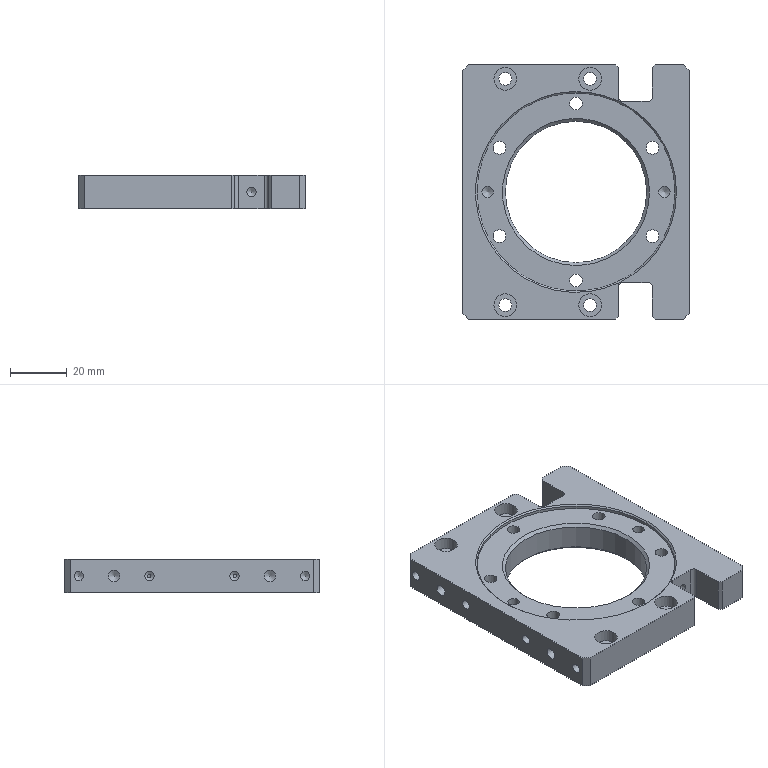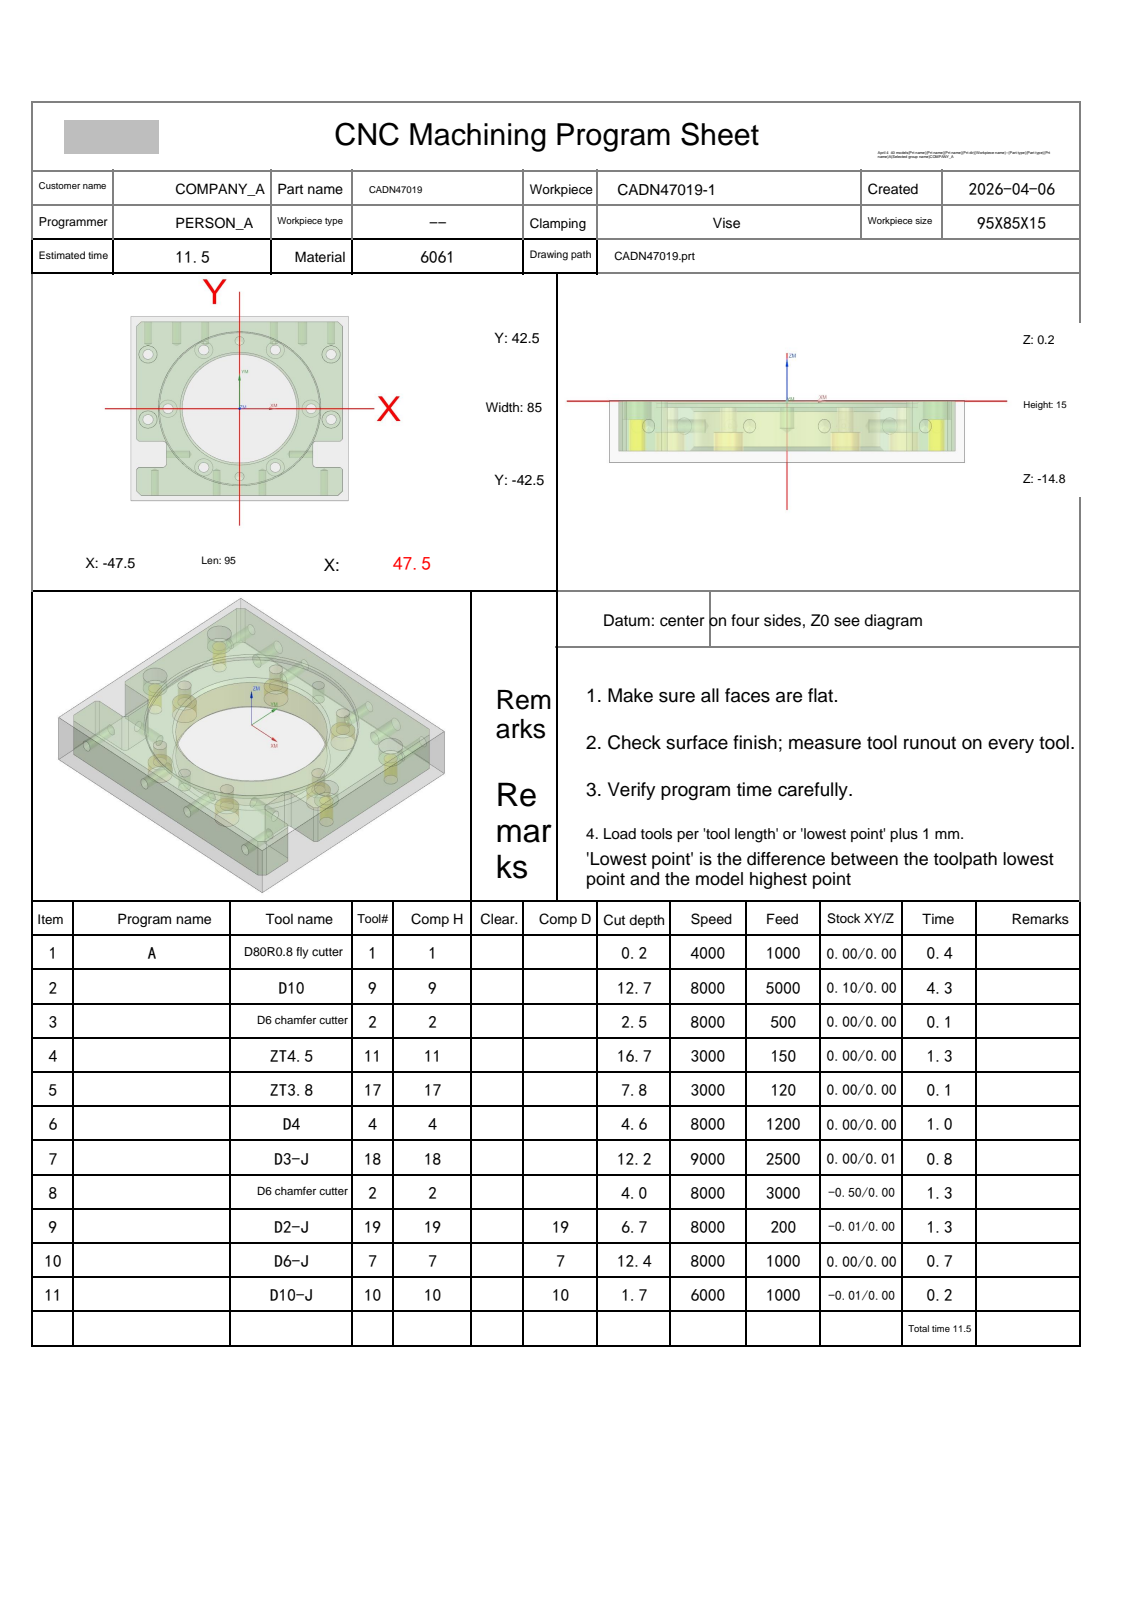NC program | NX | posted by the shop | part box 80 x 90 x 12 mm
Lines 1 to 1818 of 6628, first 1268 of 1816 lines:
%
O0001
(Machine time: 13.74 MIN)
(===Total Tool:10===)
(T1=D80R0.8 fly cutter D=80.  R=0.8  D-  H01 Z=-0.   )
(T9=D10     D=10.  R=0.   D-  H09 Z=-12.5 )
(T2=D6 chamfer cutter   D=6.   R=0.   D-  H02 Z=-3.8  )
(T11=ZT4.5  D=4.5  DR_a=118 D-  H11 Z=-16.5 )
(T17=ZT3.8  D=3.8  DR_a=118 D-  H17 Z=-7.6  )
(T4=D4      D=4.   R=0.   D4  H04 Z=-4.4  )
(T18=D3-J   D=3.   R=0.   D-  H18 Z=-11.95)
(T19=D2-J   D=2.   R=0.   D19 H19 Z=-6.5  )
(T7=D6-J    D=6.   R=0.   D7  H07 Z=-12.2 )
(T10=D10-J  D=10.  R=0.   D10 H10 Z=-1.5  )
G80 G90 G17 G49 G40
G91 G28 Z0
M01
N1 T01 M06
(D80R0.8 fly cutter  D=80. R=0.8 H=01 ce=0.00 di=0.00)
G00 G90 G54 X-90. Y26.667 M03 S4000
G43 H01 Z20.
M08
Z2.
G01 Z0.0 F1000.
X-85.
X85.
Y-26.667
X-85.
X-90.
Z2.
G00 Z20.
G91 G28 Z0.0
M05
M09
G91 G28 Z0.0
M01
N2 T09 M06
(D10  D=10. R=0. H=09 ce=0.10 di=0.00)
G00 G90 G54 X0.0 Y-45.1 M03 S8000
G43 H09 Z20.
M08
Z.5
G01 X-43. Z.416 F5000.
G02 X-46.606 Y-43.606 Z.409 I0.0 J5.1
G01 X-48.606 Y-41.606 Z.403
G02 X-50.1 Y-38. Z.395 I3.606 J3.606
G01 Y-28. Z.376
G02 X-48.606 Y-24.394 Z.368 I5.1 J0.0
G01 X-47.606 Y-23.394 Z.365
G02 X-44. Y-21.9 Z.358 I3.606 J-3.606
G01 X-37.1 Z.344
Y-20.1 Z.341
X-44. Z.327
G02 X-47.606 Y-18.606 Z.319 I0.0 J5.1
G01 X-48.606 Y-17.606 Z.317
G02 X-50.1 Y-14. Z.309 I3.606 J3.606
G01 Y38. Z.208
G02 X-48.606 Y41.606 Z.2 I5.1 J0.0
G01 X-46.606 Y43.606 Z.195
G02 X-43. Y45.1 Z.187 I3.606 J-3.606
G01 X43. Z.02
G02 X46.606 Y43.606 Z.012 I0.0 J-5.1
G01 X48.606 Y41.606 Z.006
G02 X50.1 Y38. Z-.002 I-3.606 J-3.606
G01 Y-14. Z-.103
G02 X48.606 Y-17.606 Z-.11 I-5.1 J0.0
G01 X47.606 Y-18.606 Z-.113
G02 X44.357 Y-20.087 Z-.12 I-3.606 J3.606
X44. Y-20.1 Z-.121 I-.357 J5.087
G01 X37.1 Z-.134
Y-21.9 Z-.138
X44. Z-.151
G02 X47.606 Y-23.394 Z-.159 I0.0 J-5.1
G01 X48.606 Y-24.394 Z-.162
G02 X50.1 Y-28. Z-.17 I-3.606 J-3.606
G01 Y-38. Z-.189
G02 X48.606 Y-41.606 Z-.197 I-5.1 J0.0
G01 X46.606 Y-43.606 Z-.202
G02 X43. Y-45.1 Z-.21 I-3.606 J3.606
G01 X-43. Z-.377
G02 X-46.606 Y-43.606 Z-.385 I0.0 J5.1
G01 X-48.606 Y-41.606 Z-.391
G02 X-50.1 Y-38. Z-.398 I3.606 J3.606
G01 Y-28. Z-.418
G02 X-48.606 Y-24.394 Z-.426 I5.1 J0.0
G01 X-47.606 Y-23.394 Z-.428
G02 X-44. Y-21.9 Z-.436 I3.606 J-3.606
G01 X-37.1 Z-.45
Y-20.1 Z-.453
X-44. Z-.467
G02 X-47.606 Y-18.606 Z-.474 I0.0 J5.1
G01 X-48.606 Y-17.606 Z-.477
G02 X-50.1 Y-14. Z-.485 I3.606 J3.606
G01 Y38. Z-.586
G02 X-48.606 Y41.606 Z-.594 I5.1 J0.0
G01 X-46.606 Y43.606 Z-.599
G02 X-43. Y45.1 Z-.607 I3.606 J-3.606
G01 X43. Z-.774
G02 X46.606 Y43.606 Z-.782 I0.0 J-5.1
G01 X48.606 Y41.606 Z-.788
G02 X50.1 Y38. Z-.795 I-3.606 J-3.606
G01 Y-14. Z-.896
G02 X48.606 Y-17.606 Z-.904 I-5.1 J0.0
G01 X47.606 Y-18.606 Z-.907
G02 X44.357 Y-20.087 Z-.914 I-3.606 J3.606
X44. Y-20.1 Z-.915 I-.357 J5.087
G01 X37.1 Z-.928
Y-21.9 Z-.932
X44. Z-.945
G02 X47.606 Y-23.394 Z-.953 I0.0 J-5.1
G01 X48.606 Y-24.394 Z-.956
G02 X50.1 Y-28. Z-.963 I-3.606 J-3.606
G01 Y-38. Z-.983
G02 X48.606 Y-41.606 Z-.991 I-5.1 J0.0
G01 X46.606 Y-43.606 Z-.996
G02 X43. Y-45.1 Z-1.004 I-3.606 J3.606
G01 X-43. Z-1.171
G02 X-46.606 Y-43.606 Z-1.179 I0.0 J5.1
G01 X-48.606 Y-41.606 Z-1.184
G02 X-50.1 Y-38. Z-1.192 I3.606 J3.606
G01 Y-28. Z-1.212
G02 X-48.606 Y-24.394 Z-1.219 I5.1 J0.0
G01 X-47.606 Y-23.394 Z-1.222
G02 X-44. Y-21.9 Z-1.23 I3.606 J-3.606
G01 X-37.1 Z-1.243
Y-20.1 Z-1.247
X-44. Z-1.26
G02 X-47.606 Y-18.606 Z-1.268 I0.0 J5.1
G01 X-48.606 Y-17.606 Z-1.271
G02 X-50.1 Y-14. Z-1.279 I3.606 J3.606
G01 Y38. Z-1.38
G02 X-48.606 Y41.606 Z-1.387 I5.1 J0.0
G01 X-46.606 Y43.606 Z-1.393
G02 X-43. Y45.1 Z-1.401 I3.606 J-3.606
G01 X43. Z-1.568
G02 X46.606 Y43.606 Z-1.576 I0.0 J-5.1
G01 X48.606 Y41.606 Z-1.581
G02 X50.1 Y38. Z-1.589 I-3.606 J-3.606
G01 Y-14. Z-1.69
G02 X48.606 Y-17.606 Z-1.698 I-5.1 J0.0
G01 X47.606 Y-18.606 Z-1.701
G02 X44.357 Y-20.087 Z-1.708 I-3.606 J3.606
X44. Y-20.1 Z-1.708 I-.357 J5.087
G01 X37.1 Z-1.722
Y-21.9 Z-1.725
X44. Z-1.739
G02 X47.606 Y-23.394 Z-1.747 I0.0 J-5.1
G01 X48.606 Y-24.394 Z-1.749
G02 X50.1 Y-28. Z-1.757 I-3.606 J-3.606
G01 Y-38. Z-1.777
G02 X48.606 Y-41.606 Z-1.784 I-5.1 J0.0
G01 X46.606 Y-43.606 Z-1.79
G02 X43. Y-45.1 Z-1.798 I-3.606 J3.606
G01 X-43. Z-1.965
G02 X-46.606 Y-43.606 Z-1.973 I0.0 J5.1
G01 X-48.606 Y-41.606 Z-1.978
G02 X-50.1 Y-38. Z-1.986 I3.606 J3.606
G01 Y-28. Z-2.005
G02 X-48.606 Y-24.394 Z-2.013 I5.1 J0.0
G01 X-47.606 Y-23.394 Z-2.016
G02 X-44. Y-21.9 Z-2.024 I3.606 J-3.606
G01 X-37.1 Z-2.037
Y-20.1 Z-2.041
X-44. Z-2.054
G02 X-47.606 Y-18.606 Z-2.062 I0.0 J5.1
G01 X-48.606 Y-17.606 Z-2.065
G02 X-50.1 Y-14. Z-2.072 I3.606 J3.606
G01 Y38. Z-2.173
G02 X-48.606 Y41.606 Z-2.181 I5.1 J0.0
G01 X-46.606 Y43.606 Z-2.187
G02 X-43. Y45.1 Z-2.195 I3.606 J-3.606
G01 X43. Z-2.362
G02 X46.606 Y43.606 Z-2.37 I0.0 J-5.1
G01 X48.606 Y41.606 Z-2.375
G02 X50.1 Y38. Z-2.383 I-3.606 J-3.606
G01 Y-14. Z-2.484
G02 X48.606 Y-17.606 Z-2.492 I-5.1 J0.0
G01 X47.606 Y-18.606 Z-2.494
G02 X44.357 Y-20.087 Z-2.502 I-3.606 J3.606
X44. Y-20.1 Z-2.502 I-.357 J5.087
G01 X37.1 Z-2.516
Y-21.9 Z-2.519
X44. Z-2.533
G02 X47.606 Y-23.394 Z-2.54 I0.0 J-5.1
G01 X48.606 Y-24.394 Z-2.543
G02 X50.1 Y-28. Z-2.551 I-3.606 J-3.606
G01 Y-38. Z-2.57
G02 X48.606 Y-41.606 Z-2.578 I-5.1 J0.0
G01 X46.606 Y-43.606 Z-2.584
G02 X43. Y-45.1 Z-2.591 I-3.606 J3.606
G01 X-43. Z-2.759
G02 X-46.606 Y-43.606 Z-2.766 I0.0 J5.1
G01 X-48.606 Y-41.606 Z-2.772
G02 X-50.1 Y-38. Z-2.78 I3.606 J3.606
G01 Y-28. Z-2.799
G02 X-48.606 Y-24.394 Z-2.807 I5.1 J0.0
G01 X-47.606 Y-23.394 Z-2.81
G02 X-44. Y-21.9 Z-2.817 I3.606 J-3.606
G01 X-37.1 Z-2.831
Y-20.1 Z-2.834
X-44. Z-2.848
G02 X-47.606 Y-18.606 Z-2.856 I0.0 J5.1
G01 X-48.606 Y-17.606 Z-2.858
G02 X-50.1 Y-14. Z-2.866 I3.606 J3.606
G01 Y38. Z-2.967
G02 X-48.606 Y41.606 Z-2.975 I5.1 J0.0
G01 X-46.606 Y43.606 Z-2.98
G02 X-43. Y45.1 Z-2.988 I3.606 J-3.606
G01 X43. Z-3.155
G02 X46.606 Y43.606 Z-3.163 I0.0 J-5.1
G01 X48.606 Y41.606 Z-3.169
G02 X50.1 Y38. Z-3.177 I-3.606 J-3.606
G01 Y-14. Z-3.278
G02 X48.606 Y-17.606 Z-3.285 I-5.1 J0.0
G01 X47.606 Y-18.606 Z-3.288
G02 X44.357 Y-20.087 Z-3.295 I-3.606 J3.606
X44. Y-20.1 Z-3.296 I-.357 J5.087
G01 X37.1 Z-3.309
Y-21.9 Z-3.313
X44. Z-3.326
G02 X47.606 Y-23.394 Z-3.334 I0.0 J-5.1
G01 X48.606 Y-24.394 Z-3.337
G02 X50.1 Y-28. Z-3.345 I-3.606 J-3.606
G01 Y-38. Z-3.364
G02 X48.606 Y-41.606 Z-3.372 I-5.1 J0.0
G01 X46.606 Y-43.606 Z-3.377
G02 X43. Y-45.1 Z-3.385 I-3.606 J3.606
G01 X-43. Z-3.552
G02 X-46.606 Y-43.606 Z-3.56 I0.0 J5.1
G01 X-48.606 Y-41.606 Z-3.566
G02 X-50.1 Y-38. Z-3.573 I3.606 J3.606
G01 Y-28. Z-3.593
G02 X-48.606 Y-24.394 Z-3.601 I5.1 J0.0
G01 X-47.606 Y-23.394 Z-3.603
G02 X-44. Y-21.9 Z-3.611 I3.606 J-3.606
G01 X-37.1 Z-3.625
Y-20.1 Z-3.628
X-44. Z-3.642
G02 X-47.606 Y-18.606 Z-3.649 I0.0 J5.1
G01 X-48.606 Y-17.606 Z-3.652
G02 X-50.1 Y-14. Z-3.66 I3.606 J3.606
G01 Y38. Z-3.761
G02 X-48.606 Y41.606 Z-3.769 I5.1 J0.0
G01 X-46.606 Y43.606 Z-3.774
G02 X-43. Y45.1 Z-3.782 I3.606 J-3.606
G01 X43. Z-3.949
G02 X46.606 Y43.606 Z-3.957 I0.0 J-5.1
G01 X48.606 Y41.606 Z-3.963
G02 X50.1 Y38. Z-3.97 I-3.606 J-3.606
G01 Y-14. Z-4.071
G02 X48.606 Y-17.606 Z-4.079 I-5.1 J0.0
G01 X47.606 Y-18.606 Z-4.082
G02 X44.357 Y-20.087 Z-4.089 I-3.606 J3.606
X44. Y-20.1 Z-4.09 I-.357 J5.087
G01 X37.1 Z-4.103
Y-21.9 Z-4.107
X44. Z-4.12
G02 X47.606 Y-23.394 Z-4.128 I0.0 J-5.1
G01 X48.606 Y-24.394 Z-4.131
G02 X50.1 Y-28. Z-4.138 I-3.606 J-3.606
G01 Y-38. Z-4.158
G02 X48.606 Y-41.606 Z-4.166 I-5.1 J0.0
G01 X46.606 Y-43.606 Z-4.171
G02 X43. Y-45.1 Z-4.179 I-3.606 J3.606
G01 X-43. Z-4.346
G02 X-46.606 Y-43.606 Z-4.354 I0.0 J5.1
G01 X-48.606 Y-41.606 Z-4.359
G02 X-50.1 Y-38. Z-4.367 I3.606 J3.606
G01 Y-28. Z-4.387
G02 X-48.606 Y-24.394 Z-4.394 I5.1 J0.0
G01 X-47.606 Y-23.394 Z-4.397
G02 X-44. Y-21.9 Z-4.405 I3.606 J-3.606
G01 X-37.1 Z-4.418
Y-20.1 Z-4.422
X-44. Z-4.435
G02 X-47.606 Y-18.606 Z-4.443 I0.0 J5.1
G01 X-48.606 Y-17.606 Z-4.446
G02 X-50.1 Y-14. Z-4.454 I3.606 J3.606
G01 Y38. Z-4.555
G02 X-48.606 Y41.606 Z-4.562 I5.1 J0.0
G01 X-46.606 Y43.606 Z-4.568
G02 X-43. Y45.1 Z-4.576 I3.606 J-3.606
G01 X43. Z-4.743
G02 X46.606 Y43.606 Z-4.751 I0.0 J-5.1
G01 X48.606 Y41.606 Z-4.756
G02 X50.1 Y38. Z-4.764 I-3.606 J-3.606
G01 Y-14. Z-4.865
G02 X48.606 Y-17.606 Z-4.873 I-5.1 J0.0
G01 X47.606 Y-18.606 Z-4.876
G02 X44.357 Y-20.087 Z-4.883 I-3.606 J3.606
X44. Y-20.1 Z-4.883 I-.357 J5.087
G01 X37.1 Z-4.897
Y-21.9 Z-4.9
X44. Z-4.914
G02 X47.606 Y-23.394 Z-4.922 I0.0 J-5.1
G01 X48.606 Y-24.394 Z-4.924
G02 X50.1 Y-28. Z-4.932 I-3.606 J-3.606
G01 Y-38. Z-4.952
G02 X48.606 Y-41.606 Z-4.959 I-5.1 J0.0
G01 X46.606 Y-43.606 Z-4.965
G02 X43. Y-45.1 Z-4.973 I-3.606 J3.606
G01 X-43. Z-5.14
G02 X-46.606 Y-43.606 Z-5.148 I0.0 J5.1
G01 X-48.606 Y-41.606 Z-5.153
G02 X-50.1 Y-38. Z-5.161 I3.606 J3.606
G01 Y-28. Z-5.18
G02 X-48.606 Y-24.394 Z-5.188 I5.1 J0.0
G01 X-47.606 Y-23.394 Z-5.191
G02 X-44. Y-21.9 Z-5.199 I3.606 J-3.606
G01 X-37.1 Z-5.212
Y-20.1 Z-5.216
X-44. Z-5.229
G02 X-47.606 Y-18.606 Z-5.237 I0.0 J5.1
G01 X-48.606 Y-17.606 Z-5.24
G02 X-50.1 Y-14. Z-5.247 I3.606 J3.606
G01 Y38. Z-5.348
G02 X-48.606 Y41.606 Z-5.356 I5.1 J0.0
G01 X-46.606 Y43.606 Z-5.362
G02 X-43. Y45.1 Z-5.37 I3.606 J-3.606
G01 X43. Z-5.537
G02 X46.606 Y43.606 Z-5.545 I0.0 J-5.1
G01 X48.606 Y41.606 Z-5.55
G02 X50.1 Y38. Z-5.558 I-3.606 J-3.606
G01 Y-14. Z-5.659
G02 X48.606 Y-17.606 Z-5.667 I-5.1 J0.0
G01 X47.606 Y-18.606 Z-5.669
G02 X44.357 Y-20.087 Z-5.677 I-3.606 J3.606
X44. Y-20.1 Z-5.677 I-.357 J5.087
G01 X37.1 Z-5.691
Y-21.9 Z-5.694
X44. Z-5.708
G02 X47.606 Y-23.394 Z-5.715 I0.0 J-5.1
G01 X48.606 Y-24.394 Z-5.718
G02 X50.1 Y-28. Z-5.726 I-3.606 J-3.606
G01 Y-38. Z-5.745
G02 X48.606 Y-41.606 Z-5.753 I-5.1 J0.0
G01 X46.606 Y-43.606 Z-5.759
G02 X43. Y-45.1 Z-5.766 I-3.606 J3.606
G01 X-43. Z-5.934
G02 X-46.606 Y-43.606 Z-5.941 I0.0 J5.1
G01 X-48.606 Y-41.606 Z-5.947
G02 X-50.1 Y-38. Z-5.955 I3.606 J3.606
G01 Y-28. Z-5.974
G02 X-48.606 Y-24.394 Z-5.982 I5.1 J0.0
G01 X-47.606 Y-23.394 Z-5.985
G02 X-44. Y-21.9 Z-5.992 I3.606 J-3.606
G01 X-37.1 Z-6.006
Y-20.1 Z-6.009
X-44. Z-6.023
G02 X-47.606 Y-18.606 Z-6.031 I0.0 J5.1
G01 X-48.606 Y-17.606 Z-6.033
G02 X-50.1 Y-14. Z-6.041 I3.606 J3.606
G01 Y38. Z-6.142
G02 X-48.606 Y41.606 Z-6.15 I5.1 J0.0
G01 X-46.606 Y43.606 Z-6.155
G02 X-43. Y45.1 Z-6.163 I3.606 J-3.606
G01 X43. Z-6.33
G02 X46.606 Y43.606 Z-6.338 I0.0 J-5.1
G01 X48.606 Y41.606 Z-6.344
G02 X50.1 Y38. Z-6.352 I-3.606 J-3.606
G01 Y-14. Z-6.453
G02 X48.606 Y-17.606 Z-6.46 I-5.1 J0.0
G01 X47.606 Y-18.606 Z-6.463
G02 X44.357 Y-20.087 Z-6.47 I-3.606 J3.606
X44. Y-20.1 Z-6.471 I-.357 J5.087
G01 X37.1 Z-6.484
Y-21.9 Z-6.488
X44. Z-6.501
G02 X47.606 Y-23.394 Z-6.509 I0.0 J-5.1
G01 X48.606 Y-24.394 Z-6.512
G02 X50.1 Y-28. Z-6.52 I-3.606 J-3.606
G01 Y-38. Z-6.539
G02 X48.606 Y-41.606 Z-6.547 I-5.1 J0.0
G01 X46.606 Y-43.606 Z-6.552
G02 X43. Y-45.1 Z-6.56 I-3.606 J3.606
G01 X-43. Z-6.727
G02 X-46.606 Y-43.606 Z-6.735 I0.0 J5.1
G01 X-48.606 Y-41.606 Z-6.741
G02 X-50.1 Y-38. Z-6.748 I3.606 J3.606
G01 Y-28. Z-6.768
G02 X-48.606 Y-24.394 Z-6.776 I5.1 J0.0
G01 X-47.606 Y-23.394 Z-6.778
G02 X-44. Y-21.9 Z-6.786 I3.606 J-3.606
G01 X-37.1 Z-6.8
Y-20.1 Z-6.803
X-44. Z-6.817
G02 X-47.606 Y-18.606 Z-6.824 I0.0 J5.1
G01 X-48.606 Y-17.606 Z-6.827
G02 X-50.1 Y-14. Z-6.835 I3.606 J3.606
G01 Y38. Z-6.936
G02 X-48.606 Y41.606 Z-6.944 I5.1 J0.0
G01 X-46.606 Y43.606 Z-6.949
G02 X-43. Y45.1 Z-6.957 I3.606 J-3.606
G01 X43. Z-7.124
G02 X46.606 Y43.606 Z-7.132 I0.0 J-5.1
G01 X48.606 Y41.606 Z-7.138
G02 X50.1 Y38. Z-7.145 I-3.606 J-3.606
G01 Y-14. Z-7.246
G02 X48.606 Y-17.606 Z-7.254 I-5.1 J0.0
G01 X47.606 Y-18.606 Z-7.257
G02 X44.357 Y-20.087 Z-7.264 I-3.606 J3.606
X44. Y-20.1 Z-7.265 I-.357 J5.087
G01 X37.1 Z-7.278
Y-21.9 Z-7.282
X44. Z-7.295
G02 X47.606 Y-23.394 Z-7.303 I0.0 J-5.1
G01 X48.606 Y-24.394 Z-7.306
G02 X50.1 Y-28. Z-7.313 I-3.606 J-3.606
G01 Y-38. Z-7.333
G02 X48.606 Y-41.606 Z-7.341 I-5.1 J0.0
G01 X46.606 Y-43.606 Z-7.346
G02 X43. Y-45.1 Z-7.354 I-3.606 J3.606
G01 X-43. Z-7.521
G02 X-46.606 Y-43.606 Z-7.529 I0.0 J5.1
G01 X-48.606 Y-41.606 Z-7.534
G02 X-50.1 Y-38. Z-7.542 I3.606 J3.606
G01 Y-28. Z-7.562
G02 X-48.606 Y-24.394 Z-7.569 I5.1 J0.0
G01 X-47.606 Y-23.394 Z-7.572
G02 X-44. Y-21.9 Z-7.58 I3.606 J-3.606
G01 X-37.1 Z-7.593
Y-20.1 Z-7.597
X-44. Z-7.61
G02 X-47.606 Y-18.606 Z-7.618 I0.0 J5.1
G01 X-48.606 Y-17.606 Z-7.621
G02 X-50.1 Y-14. Z-7.629 I3.606 J3.606
G01 Y38. Z-7.73
G02 X-48.606 Y41.606 Z-7.737 I5.1 J0.0
G01 X-46.606 Y43.606 Z-7.743
G02 X-43. Y45.1 Z-7.751 I3.606 J-3.606
G01 X43. Z-7.918
G02 X46.606 Y43.606 Z-7.926 I0.0 J-5.1
G01 X48.606 Y41.606 Z-7.931
G02 X50.1 Y38. Z-7.939 I-3.606 J-3.606
G01 Y-14. Z-8.04
G02 X48.606 Y-17.606 Z-8.048 I-5.1 J0.0
G01 X47.606 Y-18.606 Z-8.051
G02 X44.357 Y-20.087 Z-8.058 I-3.606 J3.606
X44. Y-20.1 Z-8.058 I-.357 J5.087
G01 X37.1 Z-8.072
Y-21.9 Z-8.075
X44. Z-8.089
G02 X47.606 Y-23.394 Z-8.097 I0.0 J-5.1
G01 X48.606 Y-24.394 Z-8.099
G02 X50.1 Y-28. Z-8.107 I-3.606 J-3.606
G01 Y-38. Z-8.127
G02 X48.606 Y-41.606 Z-8.134 I-5.1 J0.0
G01 X46.606 Y-43.606 Z-8.14
G02 X43. Y-45.1 Z-8.148 I-3.606 J3.606
G01 X-43. Z-8.315
G02 X-46.606 Y-43.606 Z-8.323 I0.0 J5.1
G01 X-48.606 Y-41.606 Z-8.328
G02 X-50.1 Y-38. Z-8.336 I3.606 J3.606
G01 Y-28. Z-8.355
G02 X-48.606 Y-24.394 Z-8.363 I5.1 J0.0
G01 X-47.606 Y-23.394 Z-8.366
G02 X-44. Y-21.9 Z-8.374 I3.606 J-3.606
G01 X-37.1 Z-8.387
Y-20.1 Z-8.391
X-44. Z-8.404
G02 X-47.606 Y-18.606 Z-8.412 I0.0 J5.1
G01 X-48.606 Y-17.606 Z-8.415
G02 X-50.1 Y-14. Z-8.422 I3.606 J3.606
G01 Y38. Z-8.523
G02 X-48.606 Y41.606 Z-8.531 I5.1 J0.0
G01 X-46.606 Y43.606 Z-8.537
G02 X-43. Y45.1 Z-8.545 I3.606 J-3.606
G01 X43. Z-8.712
G02 X46.606 Y43.606 Z-8.72 I0.0 J-5.1
G01 X48.606 Y41.606 Z-8.725
G02 X50.1 Y38. Z-8.733 I-3.606 J-3.606
G01 Y-14. Z-8.834
G02 X48.606 Y-17.606 Z-8.842 I-5.1 J0.0
G01 X47.606 Y-18.606 Z-8.844
G02 X44.357 Y-20.087 Z-8.852 I-3.606 J3.606
X44. Y-20.1 Z-8.852 I-.357 J5.087
G01 X37.1 Z-8.866
Y-21.9 Z-8.869
X44. Z-8.883
G02 X47.606 Y-23.394 Z-8.89 I0.0 J-5.1
G01 X48.606 Y-24.394 Z-8.893
G02 X50.1 Y-28. Z-8.901 I-3.606 J-3.606
G01 Y-38. Z-8.92
G02 X48.606 Y-41.606 Z-8.928 I-5.1 J0.0
G01 X46.606 Y-43.606 Z-8.934
G02 X43. Y-45.1 Z-8.941 I-3.606 J3.606
G01 X-43. Z-9.109
G02 X-46.606 Y-43.606 Z-9.116 I0.0 J5.1
G01 X-48.606 Y-41.606 Z-9.122
G02 X-50.1 Y-38. Z-9.13 I3.606 J3.606
G01 Y-28. Z-9.149
G02 X-48.606 Y-24.394 Z-9.157 I5.1 J0.0
G01 X-47.606 Y-23.394 Z-9.16
G02 X-44. Y-21.9 Z-9.167 I3.606 J-3.606
G01 X-37.1 Z-9.181
Y-20.1 Z-9.184
X-44. Z-9.198
G02 X-47.606 Y-18.606 Z-9.206 I0.0 J5.1
G01 X-48.606 Y-17.606 Z-9.208
G02 X-50.1 Y-14. Z-9.216 I3.606 J3.606
G01 Y38. Z-9.317
G02 X-48.606 Y41.606 Z-9.325 I5.1 J0.0
G01 X-46.606 Y43.606 Z-9.33
G02 X-43. Y45.1 Z-9.338 I3.606 J-3.606
G01 X43. Z-9.505
G02 X46.606 Y43.606 Z-9.513 I0.0 J-5.1
G01 X48.606 Y41.606 Z-9.519
G02 X50.1 Y38. Z-9.527 I-3.606 J-3.606
G01 Y-14. Z-9.628
G02 X48.606 Y-17.606 Z-9.635 I-5.1 J0.0
G01 X47.606 Y-18.606 Z-9.638
G02 X44.357 Y-20.087 Z-9.645 I-3.606 J3.606
X44. Y-20.1 Z-9.646 I-.357 J5.087
G01 X37.1 Z-9.659
Y-21.9 Z-9.663
X44. Z-9.676
G02 X47.606 Y-23.394 Z-9.684 I0.0 J-5.1
G01 X48.606 Y-24.394 Z-9.687
G02 X50.1 Y-28. Z-9.695 I-3.606 J-3.606
G01 Y-38. Z-9.714
G02 X48.606 Y-41.606 Z-9.722 I-5.1 J0.0
G01 X46.606 Y-43.606 Z-9.727
G02 X43. Y-45.1 Z-9.735 I-3.606 J3.606
G01 X-43. Z-9.902
G02 X-46.606 Y-43.606 Z-9.91 I0.0 J5.1
G01 X-48.606 Y-41.606 Z-9.916
G02 X-50.1 Y-38. Z-9.923 I3.606 J3.606
G01 Y-28. Z-9.943
G02 X-48.606 Y-24.394 Z-9.951 I5.1 J0.0
G01 X-47.606 Y-23.394 Z-9.953
G02 X-44. Y-21.9 Z-9.961 I3.606 J-3.606
G01 X-37.1 Z-9.975
Y-20.1 Z-9.978
X-44. Z-9.992
G02 X-47.606 Y-18.606 Z-9.999 I0.0 J5.1
G01 X-48.606 Y-17.606 Z-10.002
G02 X-50.1 Y-14. Z-10.01 I3.606 J3.606
G01 Y38. Z-10.111
G02 X-48.606 Y41.606 Z-10.119 I5.1 J0.0
G01 X-46.606 Y43.606 Z-10.124
G02 X-43. Y45.1 Z-10.132 I3.606 J-3.606
G01 X43. Z-10.299
G02 X46.606 Y43.606 Z-10.307 I0.0 J-5.1
G01 X48.606 Y41.606 Z-10.313
G02 X50.1 Y38. Z-10.32 I-3.606 J-3.606
G01 Y-14. Z-10.421
G02 X48.606 Y-17.606 Z-10.429 I-5.1 J0.0
G01 X47.606 Y-18.606 Z-10.432
G02 X44.357 Y-20.087 Z-10.439 I-3.606 J3.606
X44. Y-20.1 Z-10.44 I-.357 J5.087
G01 X37.1 Z-10.453
Y-21.9 Z-10.457
X44. Z-10.47
G02 X47.606 Y-23.394 Z-10.478 I0.0 J-5.1
G01 X48.606 Y-24.394 Z-10.481
G02 X50.1 Y-28. Z-10.488 I-3.606 J-3.606
G01 Y-38. Z-10.508
G02 X48.606 Y-41.606 Z-10.516 I-5.1 J0.0
G01 X46.606 Y-43.606 Z-10.521
G02 X43. Y-45.1 Z-10.529 I-3.606 J3.606
G01 X-43. Z-10.696
G02 X-46.606 Y-43.606 Z-10.704 I0.0 J5.1
G01 X-48.606 Y-41.606 Z-10.709
G02 X-50.1 Y-38. Z-10.717 I3.606 J3.606
G01 Y-28. Z-10.737
G02 X-48.606 Y-24.394 Z-10.744 I5.1 J0.0
G01 X-47.606 Y-23.394 Z-10.747
G02 X-44. Y-21.9 Z-10.755 I3.606 J-3.606
G01 X-37.1 Z-10.768
Y-20.1 Z-10.772
X-44. Z-10.785
G02 X-47.606 Y-18.606 Z-10.793 I0.0 J5.1
G01 X-48.606 Y-17.606 Z-10.796
G02 X-50.1 Y-14. Z-10.804 I3.606 J3.606
G01 Y38. Z-10.905
G02 X-48.606 Y41.606 Z-10.912 I5.1 J0.0
G01 X-46.606 Y43.606 Z-10.918
G02 X-43. Y45.1 Z-10.926 I3.606 J-3.606
G01 X43. Z-11.093
G02 X46.606 Y43.606 Z-11.101 I0.0 J-5.1
G01 X48.606 Y41.606 Z-11.106
G02 X50.1 Y38. Z-11.114 I-3.606 J-3.606
G01 Y-14. Z-11.215
G02 X48.606 Y-17.606 Z-11.223 I-5.1 J0.0
G01 X47.606 Y-18.606 Z-11.226
G02 X44.357 Y-20.087 Z-11.233 I-3.606 J3.606
X44. Y-20.1 Z-11.233 I-.357 J5.087
G01 X37.1 Z-11.247
Y-21.9 Z-11.25
X44. Z-11.264
G02 X47.606 Y-23.394 Z-11.272 I0.0 J-5.1
G01 X48.606 Y-24.394 Z-11.274
G02 X50.1 Y-28. Z-11.282 I-3.606 J-3.606
G01 Y-38. Z-11.302
G02 X48.606 Y-41.606 Z-11.309 I-5.1 J0.0
G01 X46.606 Y-43.606 Z-11.315
G02 X43. Y-45.1 Z-11.323 I-3.606 J3.606
G01 X-43. Z-11.49
G02 X-46.606 Y-43.606 Z-11.498 I0.0 J5.1
G01 X-48.606 Y-41.606 Z-11.503
G02 X-50.1 Y-38. Z-11.511 I3.606 J3.606
G01 Y-28. Z-11.53
G02 X-48.606 Y-24.394 Z-11.538 I5.1 J0.0
G01 X-47.606 Y-23.394 Z-11.541
G02 X-44. Y-21.9 Z-11.549 I3.606 J-3.606
G01 X-37.1 Z-11.562
Y-20.1 Z-11.566
X-44. Z-11.579
G02 X-47.606 Y-18.606 Z-11.587 I0.0 J5.1
G01 X-48.606 Y-17.606 Z-11.59
G02 X-50.1 Y-14. Z-11.597 I3.606 J3.606
G01 Y38. Z-11.698
G02 X-48.606 Y41.606 Z-11.706 I5.1 J0.0
G01 X-46.606 Y43.606 Z-11.712
G02 X-43. Y45.1 Z-11.72 I3.606 J-3.606
G01 X43. Z-11.887
G02 X46.606 Y43.606 Z-11.895 I0.0 J-5.1
G01 X48.606 Y41.606 Z-11.9
G02 X50.1 Y38. Z-11.908 I-3.606 J-3.606
G01 Y-14. Z-12.009
G02 X48.606 Y-17.606 Z-12.017 I-5.1 J0.0
G01 X47.606 Y-18.606 Z-12.019
G02 X44.357 Y-20.087 Z-12.027 I-3.606 J3.606
X44. Y-20.1 Z-12.027 I-.357 J5.087
G01 X37.1 Z-12.041
Y-21.9 Z-12.044
X44. Z-12.058
G02 X47.606 Y-23.394 Z-12.065 I0.0 J-5.1
G01 X48.606 Y-24.394 Z-12.068
G02 X50.1 Y-28. Z-12.076 I-3.606 J-3.606
G01 Y-38. Z-12.095
G02 X48.606 Y-41.606 Z-12.103 I-5.1 J0.0
G01 X46.606 Y-43.606 Z-12.109
G02 X43. Y-45.1 Z-12.116 I-3.606 J3.606
G01 X0.0 Z-12.2
X-43.
G02 X-46.606 Y-43.606 I0.0 J5.1
G01 X-48.606 Y-41.606
G02 X-50.1 Y-38. I3.606 J3.606
G01 Y-28.
G02 X-48.606 Y-24.394 I5.1 J0.0
G01 X-47.606 Y-23.394
G02 X-44. Y-21.9 I3.606 J-3.606
G01 X-37.1
Y-20.1
X-44.
G02 X-47.606 Y-18.606 I0.0 J5.1
G01 X-48.606 Y-17.606
G02 X-50.1 Y-14. I3.606 J3.606
G01 Y38.
G02 X-48.606 Y41.606 I5.1 J0.0
G01 X-46.606 Y43.606
G02 X-43. Y45.1 I3.606 J-3.606
G01 X43.
G02 X46.606 Y43.606 I0.0 J-5.1
G01 X48.606 Y41.606
G02 X50.1 Y38. I-3.606 J-3.606
G01 Y-14.
G02 X48.606 Y-17.606 I-5.1 J0.0
G01 X47.606 Y-18.606
G02 X44. Y-20.1 I-3.606 J3.606
G01 X37.1
Y-21.9
X44.
G02 X47.606 Y-23.394 I0.0 J-5.1
G01 X48.606 Y-24.394
G02 X50.1 Y-28. I-3.606 J-3.606
G01 Y-38.
G02 X48.606 Y-41.606 I-5.1 J0.0
G01 X46.606 Y-43.606
G02 X43. Y-45.1 I-3.606 J3.606
G01 X0.0
X-.5
Z-11.2
G00 Z20.
G00 G90 X3.941 Y22.227 M03 S8000
Z10.2
Z1.5
G02 X3.941 Y22.227 Z1.105 I-3.941 J2.173 F4000.
X3.941 Y22.227 Z.71 I-3.941 J2.173
X3.941 Y22.227 Z.316 I-3.941 J2.173
X3.941 Y22.227 Z-.079 I-3.941 J2.173
X3.941 Y22.227 Z-.474 I-3.941 J2.173
X-2.587 Y28.082 Z-.7 I-3.941 J2.173
G01 X0.0 Y29.9
G02 X29.9 Y0.0 I0.0 J-29.9
X0.0 Y-29.9 I-29.9 J0.0
X-29.9 Y0.0 I0.0 J29.9
X0.0 Y29.9 I29.9 J0.0
X4.977 Y29.483 I0.0 J-29.9
X5.808 Y28.564 I-.166 J-.986
G01 X6.202 Y22.722
G03 X6.899 Y21.836 I.998 J.068
G02 X22.9 Y0.0 I-6.899 J-21.836
X0.0 Y-22.9 I-22.9 J0.0
X-22.9 Y0.0 I0.0 J22.9
X0.0 Y22.9 I22.9 J0.0
X.718 Y22.889 I0.0 J-22.9
X1.588 Y22.322 I-.032 J-.999
G01 X4.89 Y15.444
G03 X5.448 Y14.938 I.901 J.433
G02 X15.9 Y0.0 I-5.448 J-14.938
X0.0 Y-15.9 I-15.9 J0.0
X-15.9 Y0.0 I0.0 J15.9
X-.505 Y15.892 I15.9 J0.0
G01 X-.473
G02 X.432 Y15.318 I0.0 J-1.
G01 X3.71 Y8.334
G03 X4.148 Y7.874 I.905 J.425
G02 X8.9 Y0.0 I-4.148 J-7.874
X0.0 Y-8.9 I-8.9 J0.0
X-8.9 Y0.0 I0.0 J8.9
X-1.924 Y8.69 I8.9 J0.0
G01 X-1.729 Y8.711
G02 X-.845 Y7.979 I0.0 J-.9
G01 X.205 Y2.459
G03 X.778 Y1.734 I.982 J.187
G02 X1.9 Y0.0 I-.778 J-1.734
X0.0 Y-1.9 I-1.9 J0.0
X-1.9 Y0.0 I0.0 J1.9
X0.0 Y1.9 I1.9 J0.0
X.316 Y1.873 I0.0 J-1.9
X.793 Y1.727 I-.316 J-1.873
G03 X3.713 Y1.088 I2.921 J6.362
X10.075 Y5.168 I0.0 J7.
G01 Z.5
G00 Z3.
G01 X3.941 Y22.227 F6000.
G00 Z.8
G02 X3.941 Y22.227 Z.405 I-3.941 J2.173 F4000.
X3.941 Y22.227 Z.01 I-3.941 J2.173
X3.941 Y22.227 Z-.384 I-3.941 J2.173
X3.941 Y22.227 Z-.779 I-3.941 J2.173
X3.941 Y22.227 Z-1.174 I-3.941 J2.173
X-2.587 Y28.082 Z-1.4 I-3.941 J2.173
G01 X0.0 Y29.9
G02 X29.9 Y0.0 I0.0 J-29.9
X0.0 Y-29.9 I-29.9 J0.0
X-29.9 Y0.0 I0.0 J29.9
X0.0 Y29.9 I29.9 J0.0
X4.977 Y29.483 I0.0 J-29.9
X5.808 Y28.564 I-.166 J-.986
G01 X6.202 Y22.722
G03 X6.899 Y21.836 I.998 J.068
G02 X22.9 Y0.0 I-6.899 J-21.836
X0.0 Y-22.9 I-22.9 J0.0
X-22.9 Y0.0 I0.0 J22.9
X0.0 Y22.9 I22.9 J0.0
X.718 Y22.889 I0.0 J-22.9
X1.588 Y22.322 I-.032 J-.999
G01 X4.89 Y15.444
G03 X5.448 Y14.938 I.901 J.433
G02 X15.9 Y0.0 I-5.448 J-14.938
X0.0 Y-15.9 I-15.9 J0.0
X-15.9 Y0.0 I0.0 J15.9
X-.505 Y15.892 I15.9 J0.0
G01 X-.473
G02 X.432 Y15.318 I0.0 J-1.
G01 X3.71 Y8.334
G03 X4.148 Y7.874 I.905 J.425
G02 X8.9 Y0.0 I-4.148 J-7.874
X0.0 Y-8.9 I-8.9 J0.0
X-8.9 Y0.0 I0.0 J8.9
X-1.924 Y8.69 I8.9 J0.0
G01 X-1.729 Y8.711
G02 X-.845 Y7.979 I0.0 J-.9
G01 X.205 Y2.459
G03 X.778 Y1.734 I.982 J.187
G02 X1.9 Y0.0 I-.778 J-1.734
X0.0 Y-1.9 I-1.9 J0.0
X-1.9 Y0.0 I0.0 J1.9
X0.0 Y1.9 I1.9 J0.0
X.316 Y1.873 I0.0 J-1.9
X.793 Y1.727 I-.316 J-1.873
G03 X3.713 Y1.088 I2.921 J6.362
X10.075 Y5.168 I0.0 J7.
G01 Z-.2
G00 Z2.3
G01 X-3.063 Y18.272 F6000.
G00 Z.1
G02 X-3.063 Y18.272 Z-.295 I3.063 J-3.296 F4000.
X-3.063 Y18.272 Z-.69 I3.063 J-3.296
X-3.063 Y18.272 Z-1.084 I3.063 J-3.296
X-3.063 Y18.272 Z-1.479 I3.063 J-3.296
X-3.063 Y18.272 Z-1.874 I3.063 J-3.296
X-2.587 Y18.658 Z-1.883 I3.063 J-3.296
G01 X0.0 Y20.476
G02 X20.476 Y0.0 I0.0 J-20.476
X0.0 Y-20.476 I-20.476 J0.0
X-20.476 Y0.0 I0.0 J20.476
X0.0 Y20.476 I20.476 J0.0
X4.95 Y19.869 I0.0 J-20.476
X5.709 Y18.898 I-.242 J-.97
G01 Y18.884
X5.623 Y12.886
Y12.872
G03 X6.165 Y11.983 I1. J0.0
G02 X13.476 Y0.0 I-6.165 J-11.983
X0.0 Y-13.476 I-13.476 J0.0
X-13.476 Y0.0 I0.0 J13.476
X0.0 Y13.476 I13.476 J0.0
G01 X.091
G02 X1.023 Y12.821 I-.007 J-1.
G01 X3.716 Y5.505
G03 X4.032 Y5.068 I.938 J.346
G02 X6.476 Y0.0 I-4.032 J-5.068
X0.0 Y-6.476 I-6.476 J0.0
X-6.476 Y0.0 I0.0 J6.476
X-1.665 Y6.258 I6.476 J0.0
X-1.408 Y6.292 I.257 J-.966
X-.439 Y5.537 I0.0 J-1.
G01 X.35 Y2.422
G03 X.876 Y1.771 I.969 J.246
G02 X1.976 Y0.0 I-.876 J-1.771
X0.0 Y-1.976 I-1.976 J0.0
X-1.976 Y0.0 I0.0 J1.976
X0.0 Y1.976 I1.976 J0.0
X.478 Y1.917 I0.0 J-1.976
X.943 Y1.737 I-.478 J-1.917
G03 X4.281 Y.889 I3.339 J6.152
X10.434 Y4.55 I0.0 J7.
G01 Z-.683
G00 Z1.6
G01 X-3.063 Y17.79 F6000.
G00 Z-.383
G02 X-3.063 Y17.79 Z-.777 I3.063 J-3.296 F4000.
X-3.063 Y17.79 Z-1.172 I3.063 J-3.296
X-3.063 Y17.79 Z-1.567 I3.063 J-3.296
X-3.063 Y17.79 Z-1.962 I3.063 J-3.296
X-3.063 Y17.79 Z-2.357 I3.063 J-3.296
X-2.587 Y18.175 Z-2.365 I3.063 J-3.296
G01 X0.0 Y19.993
G02 X19.993 Y0.0 I0.0 J-19.993
X0.0 Y-19.993 I-19.993 J0.0
X-19.993 Y0.0 I0.0 J19.993
X0.0 Y19.993 I19.993 J0.0
X4.221 Y19.543 I0.0 J-19.993
X5.007 Y18.646 I-.211 J-.977
G01 X5.518 Y12.303
G03 X6.049 Y11.499 I.997 J.081
G02 X12.993 Y0.0 I-6.049 J-11.499
X0.0 Y-12.993 I-12.993 J0.0
X-12.993 Y0.0 I0.0 J12.993
X0.0 Y12.993 I12.993 J0.0
G01 X.041
G02 X.979 Y12.331 I-.003 J-1.
G01 X3.616 Y4.967
G03 X3.905 Y4.546 I.941 J.337
G02 X5.993 Y0.0 I-3.905 J-4.546
X0.0 Y-5.993 I-5.993 J0.0
X-5.993 Y0.0 I0.0 J5.993
X-1.784 Y5.722 I5.993 J0.0
X-1.486 Y5.767 I.298 J-.955
X-.516 Y5.008 I0.0 J-1.
G01 X.249 Y1.934
G03 X.73 Y1.303 I.97 J.242
G02 X1.493 Y0.0 I-.73 J-1.303
X0.0 Y-1.493 I-1.493 J0.0
X-1.493 Y0.0 I0.0 J1.493
X0.0 Y1.493 I1.493 J0.0
X.37 Y1.447 I0.0 J-1.493
X.825 Y1.245 I-.37 J-1.447
G03 X4.689 Y.081 I3.865 J5.836
X10.526 Y3.217 I0.0 J7.
G01 Z-1.165
G00 Z1.117
G01 X-3.063 Y17.696 F6000.
G00 Z-.865
G02 X-3.063 Y17.696 Z-1.26 I3.063 J-3.296 F4000.
X-3.063 Y17.696 Z-1.655 I3.063 J-3.296
X-3.063 Y17.696 Z-2.05 I3.063 J-3.296
X-3.063 Y17.696 Z-2.444 I3.063 J-3.296
X-3.063 Y17.696 Z-2.839 I3.063 J-3.296
X-2.587 Y18.082 Z-2.848 I3.063 J-3.296
G01 X0.0 Y19.9
G02 X19.9 Y0.0 I0.0 J-19.9
X0.0 Y-19.9 I-19.9 J0.0
X-19.9 Y0.0 I0.0 J19.9
X0.0 Y19.9 I19.9 J0.0
X4.948 Y19.275 I0.0 J-19.9
X5.699 Y18.307 I-.249 J-.969
G01 Y18.285
X5.567 Y12.272
Y12.251
G03 X6.094 Y11.37 I1. J0.0
G02 X12.9 Y0.0 I-6.094 J-11.37
X0.0 Y-12.9 I-12.9 J0.0
X-12.9 Y0.0 I0.0 J12.9
X0.0 Y12.9 I12.9 J0.0
G01 X.031
G02 X.97 Y12.236 I-.003 J-1.
G01 X3.596 Y4.862
G03 X3.88 Y4.445 I.942 J.336
G02 X5.9 Y0.0 I-3.88 J-4.445
X0.0 Y-5.9 I-5.9 J0.0
X-5.9 Y0.0 I0.0 J5.9
X-1.808 Y5.616 I5.9 J0.0
X-1.502 Y5.664 I.306 J-.952
X-.531 Y4.905 I0.0 J-1.
G01 X.229 Y1.838
G03 X.699 Y1.213 I.971 J.241
G02 X1.4 Y0.0 I-.699 J-1.213
X0.0 Y-1.4 I-1.4 J0.0
X-1.4 Y0.0 I0.0 J1.4
X0.0 Y1.4 I1.4 J0.0
X.348 Y1.356 I0.0 J-1.4
X.8 Y1.149 I-.348 J-1.356
G03 X4.801 Y-.107 I4.001 J5.744
X10.545 Y2.892 I0.0 J7.
G01 Z-1.648
G00 Z.635
G01 X-3.063 Y17.696 F6000.
G00 Z-1.348
G02 X-3.063 Y17.696 Z-1.743 I3.063 J-3.296 F4000.
X-3.063 Y17.696 Z-2.137 I3.063 J-3.296
X-3.063 Y17.696 Z-2.532 I3.063 J-3.296
X-3.063 Y17.696 Z-2.927 I3.063 J-3.296
X-3.063 Y17.696 Z-3.322 I3.063 J-3.296
X-2.587 Y18.082 Z-3.33 I3.063 J-3.296
G01 X0.0 Y19.9
G02 X19.9 Y0.0 I0.0 J-19.9
X0.0 Y-19.9 I-19.9 J0.0
X-19.9 Y0.0 I0.0 J19.9
X0.0 Y19.9 I19.9 J0.0
X4.948 Y19.275 I0.0 J-19.9
X5.699 Y18.307 I-.249 J-.969
G01 Y18.285
X5.567 Y12.272
Y12.251
G03 X6.094 Y11.37 I1. J0.0
G02 X12.9 Y0.0 I-6.094 J-11.37
X0.0 Y-12.9 I-12.9 J0.0
X-12.9 Y0.0 I0.0 J12.9
X0.0 Y12.9 I12.9 J0.0
G01 X.031
G02 X.97 Y12.236 I-.003 J-1.
G01 X3.596 Y4.862
G03 X3.88 Y4.445 I.942 J.336
G02 X5.9 Y0.0 I-3.88 J-4.445
X0.0 Y-5.9 I-5.9 J0.0
X-5.9 Y0.0 I0.0 J5.9
X-1.808 Y5.616 I5.9 J0.0
X-1.502 Y5.664 I.306 J-.952
X-.531 Y4.905 I0.0 J-1.
G01 X.229 Y1.838
G03 X.699 Y1.213 I.971 J.241
G02 X1.4 Y0.0 I-.699 J-1.213
X0.0 Y-1.4 I-1.4 J0.0
X-1.4 Y0.0 I0.0 J1.4
X0.0 Y1.4 I1.4 J0.0
X.348 Y1.356 I0.0 J-1.4
X.8 Y1.149 I-.348 J-1.356
G03 X4.801 Y-.107 I4.001 J5.744
X10.545 Y2.892 I0.0 J7.
G01 Z-2.13
G00 Z.152
G01 X-3.063 Y17.696 F6000.
G00 Z-1.83
G02 X-3.063 Y17.696 Z-2.225 I3.063 J-3.296 F4000.
X-3.063 Y17.696 Z-2.62 I3.063 J-3.296
X-3.063 Y17.696 Z-3.015 I3.063 J-3.296
X-3.063 Y17.696 Z-3.41 I3.063 J-3.296
X-3.063 Y17.696 Z-3.804 I3.063 J-3.296
X-2.587 Y18.082 Z-3.813 I3.063 J-3.296
G01 X0.0 Y19.9
G02 X19.9 Y0.0 I0.0 J-19.9
X0.0 Y-19.9 I-19.9 J0.0
X-19.9 Y0.0 I0.0 J19.9
X0.0 Y19.9 I19.9 J0.0
X4.948 Y19.275 I0.0 J-19.9
X5.699 Y18.307 I-.249 J-.969
G01 Y18.285
X5.567 Y12.272
Y12.251
G03 X6.094 Y11.37 I1. J0.0
G02 X12.9 Y0.0 I-6.094 J-11.37
X0.0 Y-12.9 I-12.9 J0.0
X-12.9 Y0.0 I0.0 J12.9
X0.0 Y12.9 I12.9 J0.0
G01 X.031
G02 X.97 Y12.236 I-.003 J-1.
G01 X3.596 Y4.862
G03 X3.88 Y4.445 I.942 J.336
G02 X5.9 Y0.0 I-3.88 J-4.445
X0.0 Y-5.9 I-5.9 J0.0
X-5.9 Y0.0 I0.0 J5.9
X-1.808 Y5.616 I5.9 J0.0
X-1.502 Y5.664 I.306 J-.952
X-.531 Y4.905 I0.0 J-1.
G01 X.229 Y1.838
G03 X.699 Y1.213 I.971 J.241
G02 X1.4 Y0.0 I-.699 J-1.213
X0.0 Y-1.4 I-1.4 J0.0
X-1.4 Y0.0 I0.0 J1.4
X0.0 Y1.4 I1.4 J0.0
X.348 Y1.356 I0.0 J-1.4
X.8 Y1.149 I-.348 J-1.356
G03 X4.801 Y-.107 I4.001 J5.744
X10.545 Y2.892 I0.0 J7.
G01 Z-2.613
G00 Z-.33
G01 X-3.063 Y17.696 F6000.
G00 Z-2.313
G02 X-3.063 Y17.696 Z-2.708 I3.063 J-3.296 F4000.
X-3.063 Y17.696 Z-3.103 I3.063 J-3.296
X-3.063 Y17.696 Z-3.497 I3.063 J-3.296
X-3.063 Y17.696 Z-3.892 I3.063 J-3.296
X-3.063 Y17.696 Z-4.287 I3.063 J-3.296
X-2.587 Y18.082 Z-4.296 I3.063 J-3.296
G01 X0.0 Y19.9
G02 X19.9 Y0.0 I0.0 J-19.9
X0.0 Y-19.9 I-19.9 J0.0
X-19.9 Y0.0 I0.0 J19.9
X0.0 Y19.9 I19.9 J0.0
X4.948 Y19.275 I0.0 J-19.9
X5.699 Y18.307 I-.249 J-.969
G01 Y18.285
X5.567 Y12.272
Y12.251
G03 X6.094 Y11.37 I1. J0.0
G02 X12.9 Y0.0 I-6.094 J-11.37
X0.0 Y-12.9 I-12.9 J0.0
X-12.9 Y0.0 I0.0 J12.9
X0.0 Y12.9 I12.9 J0.0
G01 X.031
G02 X.97 Y12.236 I-.003 J-1.
G01 X3.596 Y4.862
G03 X3.88 Y4.445 I.942 J.336
G02 X5.9 Y0.0 I-3.88 J-4.445
X0.0 Y-5.9 I-5.9 J0.0
X-5.9 Y0.0 I0.0 J5.9
X-1.808 Y5.616 I5.9 J0.0
X-1.502 Y5.664 I.306 J-.952
X-.531 Y4.905 I0.0 J-1.
G01 X.229 Y1.838
G03 X.699 Y1.213 I.971 J.241
G02 X1.4 Y0.0 I-.699 J-1.213
X0.0 Y-1.4 I-1.4 J0.0
X-1.4 Y0.0 I0.0 J1.4
X0.0 Y1.4 I1.4 J0.0
X.348 Y1.356 I0.0 J-1.4
X.8 Y1.149 I-.348 J-1.356
G03 X4.801 Y-.107 I4.001 J5.744
X10.545 Y2.892 I0.0 J7.
G01 Z-3.096
G00 Z-.813
G01 X-3.063 Y17.696 F6000.
G00 Z-2.796
G02 X-3.063 Y17.696 Z-3.19 I3.063 J-3.296 F4000.
X-3.063 Y17.696 Z-3.585 I3.063 J-3.296
X-3.063 Y17.696 Z-3.98 I3.063 J-3.296
X-3.063 Y17.696 Z-4.375 I3.063 J-3.296
X-3.063 Y17.696 Z-4.77 I3.063 J-3.296
X-2.587 Y18.082 Z-4.778 I3.063 J-3.296
G01 X0.0 Y19.9
G02 X19.9 Y0.0 I0.0 J-19.9
X0.0 Y-19.9 I-19.9 J0.0
X-19.9 Y0.0 I0.0 J19.9
X0.0 Y19.9 I19.9 J0.0
X4.948 Y19.275 I0.0 J-19.9
X5.699 Y18.307 I-.249 J-.969
G01 Y18.285
X5.567 Y12.272
Y12.251
G03 X6.094 Y11.37 I1. J0.0
G02 X12.9 Y0.0 I-6.094 J-11.37
X0.0 Y-12.9 I-12.9 J0.0
X-12.9 Y0.0 I0.0 J12.9
X0.0 Y12.9 I12.9 J0.0
G01 X.031
G02 X.97 Y12.236 I-.003 J-1.
G01 X3.596 Y4.862
G03 X3.88 Y4.445 I.942 J.336
G02 X5.9 Y0.0 I-3.88 J-4.445
X0.0 Y-5.9 I-5.9 J0.0
X-5.9 Y0.0 I0.0 J5.9
X-1.808 Y5.616 I5.9 J0.0
X-1.502 Y5.664 I.306 J-.952
X-.531 Y4.905 I0.0 J-1.
G01 X.229 Y1.838
G03 X.699 Y1.213 I.971 J.241
G02 X1.4 Y0.0 I-.699 J-1.213
X0.0 Y-1.4 I-1.4 J0.0
X-1.4 Y0.0 I0.0 J1.4
X0.0 Y1.4 I1.4 J0.0
X.348 Y1.356 I0.0 J-1.4
X.8 Y1.149 I-.348 J-1.356
G03 X4.801 Y-.107 I4.001 J5.744
X10.545 Y2.892 I0.0 J7.
G01 Z-3.578
G00 Z-1.296
G01 X-3.063 Y17.696 F6000.
G00 Z-3.278
G02 X-3.063 Y17.696 Z-3.673 I3.063 J-3.296 F4000.
X-3.063 Y17.696 Z-4.068 I3.063 J-3.296
X-3.063 Y17.696 Z-4.463 I3.063 J-3.296
X-3.063 Y17.696 Z-4.858 I3.063 J-3.296
X-3.063 Y17.696 Z-5.252 I3.063 J-3.296
X-2.587 Y18.082 Z-5.261 I3.063 J-3.296
G01 X0.0 Y19.9
G02 X19.9 Y0.0 I0.0 J-19.9
X0.0 Y-19.9 I-19.9 J0.0
X-19.9 Y0.0 I0.0 J19.9
X0.0 Y19.9 I19.9 J0.0
X4.948 Y19.275 I0.0 J-19.9
X5.699 Y18.307 I-.249 J-.969
G01 Y18.285
X5.567 Y12.272
Y12.251
G03 X6.094 Y11.37 I1. J0.0
G02 X12.9 Y0.0 I-6.094 J-11.37
X0.0 Y-12.9 I-12.9 J0.0
X-12.9 Y0.0 I0.0 J12.9
X0.0 Y12.9 I12.9 J0.0
G01 X.031
G02 X.97 Y12.236 I-.003 J-1.
G01 X3.596 Y4.862
G03 X3.88 Y4.445 I.942 J.336
G02 X5.9 Y0.0 I-3.88 J-4.445
X0.0 Y-5.9 I-5.9 J0.0
X-5.9 Y0.0 I0.0 J5.9
X-1.808 Y5.616 I5.9 J0.0
X-1.502 Y5.664 I.306 J-.952
X-.531 Y4.905 I0.0 J-1.
G01 X.229 Y1.838
G03 X.699 Y1.213 I.971 J.241
G02 X1.4 Y0.0 I-.699 J-1.213
X0.0 Y-1.4 I-1.4 J0.0
X-1.4 Y0.0 I0.0 J1.4
X0.0 Y1.4 I1.4 J0.0
X.348 Y1.356 I0.0 J-1.4
X.8 Y1.149 I-.348 J-1.356
G03 X4.801 Y-.107 I4.001 J5.744
X10.545 Y2.892 I0.0 J7.
G01 Z-4.061
G00 Z-1.778
G01 X-3.063 Y17.696 F6000.
G00 Z-3.761
G02 X-3.063 Y17.696 Z-4.156 I3.063 J-3.296 F4000.
X-3.063 Y17.696 Z-4.55 I3.063 J-3.296
X-3.063 Y17.696 Z-4.945 I3.063 J-3.296
X-3.063 Y17.696 Z-5.34 I3.063 J-3.296
X-3.063 Y17.696 Z-5.735 I3.063 J-3.296
X-2.587 Y18.082 Z-5.743 I3.063 J-3.296
G01 X0.0 Y19.9
G02 X19.9 Y0.0 I0.0 J-19.9
X0.0 Y-19.9 I-19.9 J0.0
X-19.9 Y0.0 I0.0 J19.9
X0.0 Y19.9 I19.9 J0.0
X4.948 Y19.275 I0.0 J-19.9
X5.699 Y18.307 I-.249 J-.969
G01 Y18.285
X5.567 Y12.272
Y12.251
G03 X6.094 Y11.37 I1. J0.0
G02 X12.9 Y0.0 I-6.094 J-11.37
X0.0 Y-12.9 I-12.9 J0.0
X-12.9 Y0.0 I0.0 J12.9
X0.0 Y12.9 I12.9 J0.0
G01 X.031
G02 X.97 Y12.236 I-.003 J-1.
G01 X3.596 Y4.862
G03 X3.88 Y4.445 I.942 J.336
G02 X5.9 Y0.0 I-3.88 J-4.445
X0.0 Y-5.9 I-5.9 J0.0
X-5.9 Y0.0 I0.0 J5.9
X-1.808 Y5.616 I5.9 J0.0
X-1.502 Y5.664 I.306 J-.952
X-.531 Y4.905 I0.0 J-1.
G01 X.229 Y1.838
G03 X.699 Y1.213 I.971 J.241
G02 X1.4 Y0.0 I-.699 J-1.213
X0.0 Y-1.4 I-1.4 J0.0
X-1.4 Y0.0 I0.0 J1.4
X0.0 Y1.4 I1.4 J0.0
X.348 Y1.356 I0.0 J-1.4
X.8 Y1.149 I-.348 J-1.356
G03 X4.801 Y-.107 I4.001 J5.744
X10.545 Y2.892 I0.0 J7.
G01 Z-4.543
G00 Z-2.261
G01 X-3.063 Y17.696 F6000.
G00 Z-4.243
G02 X-3.063 Y17.696 Z-4.638 I3.063 J-3.296 F4000.
X-3.063 Y17.696 Z-5.033 I3.063 J-3.296
X-3.063 Y17.696 Z-5.428 I3.063 J-3.296
X-3.063 Y17.696 Z-5.823 I3.063 J-3.296
X-3.063 Y17.696 Z-6.218 I3.063 J-3.296
X-2.587 Y18.082 Z-6.226 I3.063 J-3.296
G01 X0.0 Y19.9
G02 X19.9 Y0.0 I0.0 J-19.9
X0.0 Y-19.9 I-19.9 J0.0
X-19.9 Y0.0 I0.0 J19.9
X0.0 Y19.9 I19.9 J0.0
X4.948 Y19.275 I0.0 J-19.9
X5.699 Y18.307 I-.249 J-.969
G01 Y18.285
X5.567 Y12.272
Y12.251
G03 X6.094 Y11.37 I1. J0.0
G02 X12.9 Y0.0 I-6.094 J-11.37
X0.0 Y-12.9 I-12.9 J0.0
X-12.9 Y0.0 I0.0 J12.9
X0.0 Y12.9 I12.9 J0.0
G01 X.031
G02 X.97 Y12.236 I-.003 J-1.
G01 X3.596 Y4.862
G03 X3.88 Y4.445 I.942 J.336
G02 X5.9 Y0.0 I-3.88 J-4.445
X0.0 Y-5.9 I-5.9 J0.0
X-5.9 Y0.0 I0.0 J5.9
X-1.808 Y5.616 I5.9 J0.0
X-1.502 Y5.664 I.306 J-.952
X-.531 Y4.905 I0.0 J-1.
G01 X.229 Y1.838
G03 X.699 Y1.213 I.971 J.241
G02 X1.4 Y0.0 I-.699 J-1.213
X0.0 Y-1.4 I-1.4 J0.0
X-1.4 Y0.0 I0.0 J1.4
X0.0 Y1.4 I1.4 J0.0
X.348 Y1.356 I0.0 J-1.4
X.8 Y1.149 I-.348 J-1.356
G03 X4.801 Y-.107 I4.001 J5.744
X10.545 Y2.892 I0.0 J7.
G01 Z-5.026
G00 Z-2.743
G01 X-3.063 Y17.696 F6000.
G00 Z-4.726
G02 X-3.063 Y17.696 Z-5.121 I3.063 J-3.296 F4000.
X-3.063 Y17.696 Z-5.516 I3.063 J-3.296
X-3.063 Y17.696 Z-5.911 I3.063 J-3.296
X-3.063 Y17.696 Z-6.305 I3.063 J-3.296
X-3.063 Y17.696 Z-6.7 I3.063 J-3.296
X-2.587 Y18.082 Z-6.709 I3.063 J-3.296
G01 X0.0 Y19.9
G02 X19.9 Y0.0 I0.0 J-19.9
X0.0 Y-19.9 I-19.9 J0.0
X-19.9 Y0.0 I0.0 J19.9
X0.0 Y19.9 I19.9 J0.0
X4.948 Y19.275 I0.0 J-19.9
X5.699 Y18.307 I-.249 J-.969
G01 Y18.285
X5.567 Y12.272
Y12.251
G03 X6.094 Y11.37 I1. J0.0
G02 X12.9 Y0.0 I-6.094 J-11.37
X0.0 Y-12.9 I-12.9 J0.0
X-12.9 Y0.0 I0.0 J12.9
X0.0 Y12.9 I12.9 J0.0
G01 X.031
G02 X.97 Y12.236 I-.003 J-1.
G01 X3.596 Y4.862
G03 X3.88 Y4.445 I.942 J.336
G02 X5.9 Y0.0 I-3.88 J-4.445
X0.0 Y-5.9 I-5.9 J0.0
X-5.9 Y0.0 I0.0 J5.9
X-1.808 Y5.616 I5.9 J0.0
X-1.502 Y5.664 I.306 J-.952
X-.531 Y4.905 I0.0 J-1.
G01 X.229 Y1.838
G03 X.699 Y1.213 I.971 J.241
G02 X1.4 Y0.0 I-.699 J-1.213
X0.0 Y-1.4 I-1.4 J0.0
X-1.4 Y0.0 I0.0 J1.4
X0.0 Y1.4 I1.4 J0.0
X.348 Y1.356 I0.0 J-1.4
X.8 Y1.149 I-.348 J-1.356
G03 X4.801 Y-.107 I4.001 J5.744